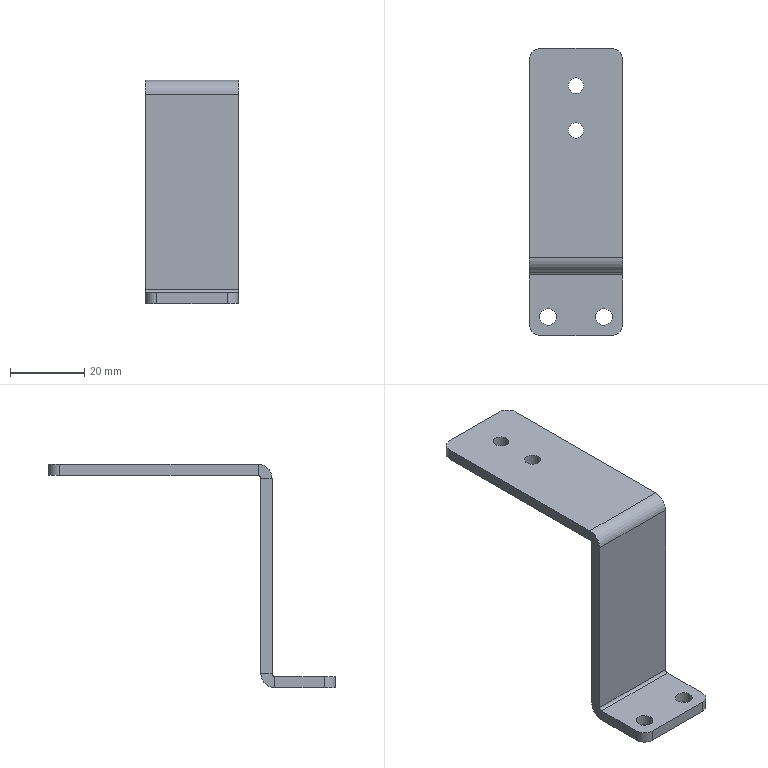Part | SolidWorks | features EdgeFlange 2, HoleWzd 2, Fillet 1, FlatPattern 1, SMBaseFlange 1, SheetMetal 1 | 1 solid | 34 faces | box 25 x 77 x 60 mm | volume 9704 mm3 | plane 18 | cylinder 16 | commonest cylinder face diameters 4.2 x4 4.5 x4 6 x4 1.473 x2 7.473 x2
STEP:
#1=CARTESIAN_POINT('',(2.1,57.,54.));
#2=VERTEX_POINT('',#1);
#3=CARTESIAN_POINT('',(-2.1,57.,54.));
#4=VERTEX_POINT('',#3);
#5=CARTESIAN_POINT('',(0.,57.,54.));
#6=DIRECTION('',(0.,0.,-1.));
#7=DIRECTION('',(-1.,0.,0.));
#8=AXIS2_PLACEMENT_3D('',#5,#6,#7);
#9=CIRCLE('',#8,2.1);
#10=EDGE_CURVE('',#2,#4,#9,.T.);
#11=ORIENTED_EDGE('',*,*,#10,.T.);
#12=CARTESIAN_POINT('',(-2.1,57.,57.));
#13=VERTEX_POINT('',#12);
#14=CARTESIAN_POINT('',(-2.1,57.,57.));
#15=DIRECTION('',(0.,0.,1.));
#16=VECTOR('',#15,1000.);
#17=LINE('',#14,#16);
#18=EDGE_CURVE('',#4,#13,#17,.T.);
#19=ORIENTED_EDGE('',*,*,#18,.T.);
#20=CARTESIAN_POINT('',(2.1,57.,57.));
#21=VERTEX_POINT('',#20);
#22=CARTESIAN_POINT('',(0.,57.,57.));
#23=DIRECTION('',(0.,0.,1.));
#24=DIRECTION('',(1.,0.,0.));
#25=AXIS2_PLACEMENT_3D('',#22,#23,#24);
#26=CIRCLE('',#25,2.1);
#27=EDGE_CURVE('',#13,#21,#26,.T.);
#28=ORIENTED_EDGE('',*,*,#27,.T.);
#29=CARTESIAN_POINT('',(2.1,57.,57.));
#30=DIRECTION('',(0.,0.,1.));
#31=VECTOR('',#30,1000.);
#32=LINE('',#29,#31);
#33=EDGE_CURVE('',#2,#21,#32,.T.);
#34=ORIENTED_EDGE('',*,*,#33,.F.);
#35=EDGE_LOOP('',(#11,#19,#28,#34));
#36=FACE_OUTER_BOUND('',#35,.T.);
#37=CARTESIAN_POINT('',(0.,57.,57.));
#38=DIRECTION('',(0.,0.,1.));
#39=DIRECTION('',(1.,0.,0.));
#40=AXIS2_PLACEMENT_3D('',#37,#38,#39);
#41=CYLINDRICAL_SURFACE('',#40,2.1);
#42=ADVANCED_FACE('',(#36),#41,.F.);
#43=CARTESIAN_POINT('',(2.1,45.,54.));
#44=VERTEX_POINT('',#43);
#45=CARTESIAN_POINT('',(-2.1,45.,54.));
#46=VERTEX_POINT('',#45);
#47=CARTESIAN_POINT('',(0.,45.,54.));
#48=DIRECTION('',(0.,0.,-1.));
#49=DIRECTION('',(-1.,0.,0.));
#50=AXIS2_PLACEMENT_3D('',#47,#48,#49);
#51=CIRCLE('',#50,2.1);
#52=EDGE_CURVE('',#44,#46,#51,.T.);
#53=ORIENTED_EDGE('',*,*,#52,.T.);
#54=CARTESIAN_POINT('',(-2.1,45.,57.));
#55=VERTEX_POINT('',#54);
#56=CARTESIAN_POINT('',(-2.1,45.,57.));
#57=DIRECTION('',(0.,0.,1.));
#58=VECTOR('',#57,1000.);
#59=LINE('',#56,#58);
#60=EDGE_CURVE('',#46,#55,#59,.T.);
#61=ORIENTED_EDGE('',*,*,#60,.T.);
#62=CARTESIAN_POINT('',(2.1,45.,57.));
#63=VERTEX_POINT('',#62);
#64=CARTESIAN_POINT('',(0.,45.,57.));
#65=DIRECTION('',(0.,0.,1.));
#66=DIRECTION('',(1.,0.,0.));
#67=AXIS2_PLACEMENT_3D('',#64,#65,#66);
#68=CIRCLE('',#67,2.1);
#69=EDGE_CURVE('',#55,#63,#68,.T.);
#70=ORIENTED_EDGE('',*,*,#69,.T.);
#71=CARTESIAN_POINT('',(2.1,45.,57.));
#72=DIRECTION('',(0.,0.,1.));
#73=VECTOR('',#72,1000.);
#74=LINE('',#71,#73);
#75=EDGE_CURVE('',#44,#63,#74,.T.);
#76=ORIENTED_EDGE('',*,*,#75,.F.);
#77=EDGE_LOOP('',(#53,#61,#70,#76));
#78=FACE_OUTER_BOUND('',#77,.T.);
#79=CARTESIAN_POINT('',(0.,45.,57.));
#80=DIRECTION('',(0.,0.,1.));
#81=DIRECTION('',(1.,0.,0.));
#82=AXIS2_PLACEMENT_3D('',#79,#80,#81);
#83=CYLINDRICAL_SURFACE('',#82,2.1);
#84=ADVANCED_FACE('',(#78),#83,.F.);
#85=CARTESIAN_POINT('',(-9.75,-5.,-3.));
#86=VERTEX_POINT('',#85);
#87=CARTESIAN_POINT('',(-5.25,-5.,-3.));
#88=VERTEX_POINT('',#87);
#89=CARTESIAN_POINT('',(-7.5,-5.,-3.));
#90=DIRECTION('',(0.,0.,1.));
#91=DIRECTION('',(1.,0.,0.));
#92=AXIS2_PLACEMENT_3D('',#89,#90,#91);
#93=CIRCLE('',#92,2.25);
#94=EDGE_CURVE('',#86,#88,#93,.T.);
#95=ORIENTED_EDGE('',*,*,#94,.F.);
#96=CARTESIAN_POINT('',(-9.75,-5.,0.));
#97=VERTEX_POINT('',#96);
#98=CARTESIAN_POINT('',(-9.75,-5.,0.));
#99=DIRECTION('',(0.,0.,1.));
#100=VECTOR('',#99,1000.);
#101=LINE('',#98,#100);
#102=EDGE_CURVE('',#86,#97,#101,.T.);
#103=ORIENTED_EDGE('',*,*,#102,.T.);
#104=CARTESIAN_POINT('',(-5.25,-5.,0.));
#105=VERTEX_POINT('',#104);
#106=CARTESIAN_POINT('',(-7.5,-5.,0.));
#107=DIRECTION('',(0.,0.,1.));
#108=DIRECTION('',(1.,0.,0.));
#109=AXIS2_PLACEMENT_3D('',#106,#107,#108);
#110=CIRCLE('',#109,2.25);
#111=EDGE_CURVE('',#97,#105,#110,.T.);
#112=ORIENTED_EDGE('',*,*,#111,.T.);
#113=CARTESIAN_POINT('',(-5.25,-5.,0.));
#114=DIRECTION('',(0.,0.,1.));
#115=VECTOR('',#114,1000.);
#116=LINE('',#113,#115);
#117=EDGE_CURVE('',#88,#105,#116,.T.);
#118=ORIENTED_EDGE('',*,*,#117,.F.);
#119=EDGE_LOOP('',(#95,#103,#112,#118));
#120=FACE_OUTER_BOUND('',#119,.T.);
#121=CARTESIAN_POINT('',(-7.5,-5.,0.));
#122=DIRECTION('',(0.,0.,1.));
#123=DIRECTION('',(1.,0.,0.));
#124=AXIS2_PLACEMENT_3D('',#121,#122,#123);
#125=CYLINDRICAL_SURFACE('',#124,2.25);
#126=ADVANCED_FACE('',(#120),#125,.F.);
#127=CARTESIAN_POINT('',(5.25,-5.,-3.));
#128=VERTEX_POINT('',#127);
#129=CARTESIAN_POINT('',(9.75,-5.,-3.));
#130=VERTEX_POINT('',#129);
#131=CARTESIAN_POINT('',(7.5,-5.,-3.));
#132=DIRECTION('',(0.,0.,1.));
#133=DIRECTION('',(1.,0.,0.));
#134=AXIS2_PLACEMENT_3D('',#131,#132,#133);
#135=CIRCLE('',#134,2.25);
#136=EDGE_CURVE('',#128,#130,#135,.T.);
#137=ORIENTED_EDGE('',*,*,#136,.F.);
#138=CARTESIAN_POINT('',(5.25,-5.,0.));
#139=VERTEX_POINT('',#138);
#140=CARTESIAN_POINT('',(5.25,-5.,0.));
#141=DIRECTION('',(0.,0.,1.));
#142=VECTOR('',#141,1000.);
#143=LINE('',#140,#142);
#144=EDGE_CURVE('',#128,#139,#143,.T.);
#145=ORIENTED_EDGE('',*,*,#144,.T.);
#146=CARTESIAN_POINT('',(9.75,-5.,0.));
#147=VERTEX_POINT('',#146);
#148=CARTESIAN_POINT('',(7.5,-5.,0.));
#149=DIRECTION('',(0.,0.,1.));
#150=DIRECTION('',(1.,0.,0.));
#151=AXIS2_PLACEMENT_3D('',#148,#149,#150);
#152=CIRCLE('',#151,2.25);
#153=EDGE_CURVE('',#139,#147,#152,.T.);
#154=ORIENTED_EDGE('',*,*,#153,.T.);
#155=CARTESIAN_POINT('',(9.75,-5.,0.));
#156=DIRECTION('',(0.,0.,1.));
#157=VECTOR('',#156,1000.);
#158=LINE('',#155,#157);
#159=EDGE_CURVE('',#130,#147,#158,.T.);
#160=ORIENTED_EDGE('',*,*,#159,.F.);
#161=EDGE_LOOP('',(#137,#145,#154,#160));
#162=FACE_OUTER_BOUND('',#161,.T.);
#163=CARTESIAN_POINT('',(7.5,-5.,0.));
#164=DIRECTION('',(0.,0.,1.));
#165=DIRECTION('',(1.,0.,0.));
#166=AXIS2_PLACEMENT_3D('',#163,#164,#165);
#167=CYLINDRICAL_SURFACE('',#166,2.25);
#168=ADVANCED_FACE('',(#162),#167,.F.);
#169=CARTESIAN_POINT('',(12.5,10.,53.263));
#170=VERTEX_POINT('',#169);
#171=CARTESIAN_POINT('',(12.5,7.,53.263));
#172=VERTEX_POINT('',#171);
#173=CARTESIAN_POINT('',(12.5,10.,53.263));
#174=DIRECTION('',(0.,-1.,0.));
#175=VECTOR('',#174,1000.);
#176=LINE('',#173,#175);
#177=EDGE_CURVE('',#170,#172,#176,.T.);
#178=ORIENTED_EDGE('',*,*,#177,.T.);
#179=CARTESIAN_POINT('',(12.5,7.,0.7366));
#180=VERTEX_POINT('',#179);
#181=CARTESIAN_POINT('',(12.5,7.,0.));
#182=DIRECTION('',(0.,0.,-1.));
#183=VECTOR('',#182,1000.);
#184=LINE('',#181,#183);
#185=EDGE_CURVE('',#172,#180,#184,.T.);
#186=ORIENTED_EDGE('',*,*,#185,.T.);
#187=CARTESIAN_POINT('',(12.5,10.,0.7366));
#188=VERTEX_POINT('',#187);
#189=CARTESIAN_POINT('',(12.5,10.,0.7366));
#190=DIRECTION('',(0.,1.,0.));
#191=VECTOR('',#190,1000.);
#192=LINE('',#189,#191);
#193=EDGE_CURVE('',#180,#188,#192,.T.);
#194=ORIENTED_EDGE('',*,*,#193,.T.);
#195=CARTESIAN_POINT('',(12.5,10.,0.));
#196=DIRECTION('',(0.,0.,-1.));
#197=VECTOR('',#196,1000.);
#198=LINE('',#195,#197);
#199=EDGE_CURVE('',#170,#188,#198,.T.);
#200=ORIENTED_EDGE('',*,*,#199,.F.);
#201=EDGE_LOOP('',(#178,#186,#194,#200));
#202=FACE_OUTER_BOUND('',#201,.T.);
#203=CARTESIAN_POINT('',(12.5,10.,0.));
#204=DIRECTION('',(-1.,0.,0.));
#205=DIRECTION('',(0.,0.,1.));
#206=AXIS2_PLACEMENT_3D('',#203,#204,#205);
#207=PLANE('',#206);
#208=ADVANCED_FACE('',(#202),#207,.F.);
#209=CARTESIAN_POINT('',(-12.5,10.,53.263));
#210=VERTEX_POINT('',#209);
#211=CARTESIAN_POINT('',(-12.5,7.,53.263));
#212=VERTEX_POINT('',#211);
#213=CARTESIAN_POINT('',(-12.5,10.,53.263));
#214=DIRECTION('',(0.,-1.,0.));
#215=VECTOR('',#214,1000.);
#216=LINE('',#213,#215);
#217=EDGE_CURVE('',#210,#212,#216,.T.);
#218=ORIENTED_EDGE('',*,*,#217,.F.);
#219=CARTESIAN_POINT('',(-12.5,10.,0.7366));
#220=VERTEX_POINT('',#219);
#221=CARTESIAN_POINT('',(-12.5,10.,0.));
#222=DIRECTION('',(0.,0.,1.));
#223=VECTOR('',#222,1000.);
#224=LINE('',#221,#223);
#225=EDGE_CURVE('',#220,#210,#224,.T.);
#226=ORIENTED_EDGE('',*,*,#225,.F.);
#227=CARTESIAN_POINT('',(-12.5,7.,0.7366));
#228=VERTEX_POINT('',#227);
#229=CARTESIAN_POINT('',(-12.5,7.,0.7366));
#230=DIRECTION('',(0.,1.,0.));
#231=VECTOR('',#230,1000.);
#232=LINE('',#229,#231);
#233=EDGE_CURVE('',#228,#220,#232,.T.);
#234=ORIENTED_EDGE('',*,*,#233,.F.);
#235=CARTESIAN_POINT('',(-12.5,7.,57.));
#236=DIRECTION('',(0.,0.,1.));
#237=VECTOR('',#236,1000.);
#238=LINE('',#235,#237);
#239=EDGE_CURVE('',#228,#212,#238,.T.);
#240=ORIENTED_EDGE('',*,*,#239,.T.);
#241=EDGE_LOOP('',(#218,#226,#234,#240));
#242=FACE_OUTER_BOUND('',#241,.T.);
#243=CARTESIAN_POINT('',(-12.5,10.,57.));
#244=DIRECTION('',(1.,0.,0.));
#245=DIRECTION('',(0.,0.,-1.));
#246=AXIS2_PLACEMENT_3D('',#243,#244,#245);
#247=PLANE('',#246);
#248=ADVANCED_FACE('',(#242),#247,.F.);
#249=CARTESIAN_POINT('',(12.5,10.,53.263));
#250=DIRECTION('',(-1.,0.,0.));
#251=VECTOR('',#250,1000.);
#252=LINE('',#249,#251);
#253=EDGE_CURVE('',#170,#210,#252,.T.);
#254=ORIENTED_EDGE('',*,*,#253,.F.);
#255=ORIENTED_EDGE('',*,*,#199,.T.);
#256=CARTESIAN_POINT('',(12.5,10.,0.7366));
#257=DIRECTION('',(1.,0.,0.));
#258=VECTOR('',#257,1000.);
#259=LINE('',#256,#258);
#260=EDGE_CURVE('',#220,#188,#259,.T.);
#261=ORIENTED_EDGE('',*,*,#260,.F.);
#262=ORIENTED_EDGE('',*,*,#225,.T.);
#263=EDGE_LOOP('',(#254,#255,#261,#262));
#264=FACE_OUTER_BOUND('',#263,.T.);
#265=CARTESIAN_POINT('',(0.,10.,0.));
#266=DIRECTION('',(0.,-1.,0.));
#267=DIRECTION('',(0.,0.,-1.));
#268=AXIS2_PLACEMENT_3D('',#265,#266,#267);
#269=PLANE('',#268);
#270=ADVANCED_FACE('',(#264),#269,.F.);
#271=ORIENTED_EDGE('',*,*,#185,.F.);
#272=CARTESIAN_POINT('',(12.5,7.,53.263));
#273=DIRECTION('',(-1.,0.,0.));
#274=VECTOR('',#273,1000.);
#275=LINE('',#272,#274);
#276=EDGE_CURVE('',#172,#212,#275,.T.);
#277=ORIENTED_EDGE('',*,*,#276,.T.);
#278=ORIENTED_EDGE('',*,*,#239,.F.);
#279=CARTESIAN_POINT('',(12.5,7.,0.7366));
#280=DIRECTION('',(-1.,0.,0.));
#281=VECTOR('',#280,1000.);
#282=LINE('',#279,#281);
#283=EDGE_CURVE('',#180,#228,#282,.T.);
#284=ORIENTED_EDGE('',*,*,#283,.F.);
#285=EDGE_LOOP('',(#271,#277,#278,#284));
#286=FACE_OUTER_BOUND('',#285,.T.);
#287=CARTESIAN_POINT('',(0.,7.,0.));
#288=DIRECTION('',(0.,-1.,0.));
#289=DIRECTION('',(0.,0.,-1.));
#290=AXIS2_PLACEMENT_3D('',#287,#288,#289);
#291=PLANE('',#290);
#292=ADVANCED_FACE('',(#286),#291,.T.);
#293=CARTESIAN_POINT('',(-12.5,6.263,-3.));
#294=VERTEX_POINT('',#293);
#295=CARTESIAN_POINT('',(-12.5,-7.,-3.));
#296=VERTEX_POINT('',#295);
#297=CARTESIAN_POINT('',(-12.5,10.,-3.));
#298=DIRECTION('',(0.,-1.,0.));
#299=VECTOR('',#298,1000.);
#300=LINE('',#297,#299);
#301=EDGE_CURVE('',#294,#296,#300,.T.);
#302=ORIENTED_EDGE('',*,*,#301,.T.);
#303=CARTESIAN_POINT('',(-12.5,-7.,0.));
#304=VERTEX_POINT('',#303);
#305=CARTESIAN_POINT('',(-12.5,-7.,-3.));
#306=DIRECTION('',(0.,0.,1.));
#307=VECTOR('',#306,1000.);
#308=LINE('',#305,#307);
#309=EDGE_CURVE('',#296,#304,#308,.T.);
#310=ORIENTED_EDGE('',*,*,#309,.T.);
#311=CARTESIAN_POINT('',(-12.5,6.263,0.));
#312=VERTEX_POINT('',#311);
#313=CARTESIAN_POINT('',(-12.5,10.,0.));
#314=DIRECTION('',(0.,-1.,0.));
#315=VECTOR('',#314,1000.);
#316=LINE('',#313,#315);
#317=EDGE_CURVE('',#312,#304,#316,.T.);
#318=ORIENTED_EDGE('',*,*,#317,.F.);
#319=CARTESIAN_POINT('',(-12.5,6.263,0.));
#320=DIRECTION('',(0.,0.,-1.));
#321=VECTOR('',#320,1000.);
#322=LINE('',#319,#321);
#323=EDGE_CURVE('',#312,#294,#322,.T.);
#324=ORIENTED_EDGE('',*,*,#323,.T.);
#325=EDGE_LOOP('',(#302,#310,#318,#324));
#326=FACE_OUTER_BOUND('',#325,.T.);
#327=CARTESIAN_POINT('',(-12.5,10.,-3.));
#328=DIRECTION('',(-1.,0.,0.));
#329=DIRECTION('',(0.,-1.,0.));
#330=AXIS2_PLACEMENT_3D('',#327,#328,#329);
#331=PLANE('',#330);
#332=ADVANCED_FACE('',(#326),#331,.T.);
#333=CARTESIAN_POINT('',(-7.5,-5.,-3.));
#334=DIRECTION('',(0.,0.,1.));
#335=DIRECTION('',(1.,0.,0.));
#336=AXIS2_PLACEMENT_3D('',#333,#334,#335);
#337=CIRCLE('',#336,2.25);
#338=EDGE_CURVE('',#88,#86,#337,.T.);
#339=ORIENTED_EDGE('',*,*,#338,.T.);
#340=ORIENTED_EDGE('',*,*,#94,.T.);
#341=EDGE_LOOP('',(#339,#340));
#342=FACE_BOUND('',#341,.T.);
#343=CARTESIAN_POINT('',(7.5,-5.,-3.));
#344=DIRECTION('',(0.,0.,1.));
#345=DIRECTION('',(1.,0.,0.));
#346=AXIS2_PLACEMENT_3D('',#343,#344,#345);
#347=CIRCLE('',#346,2.25);
#348=EDGE_CURVE('',#130,#128,#347,.T.);
#349=ORIENTED_EDGE('',*,*,#348,.T.);
#350=ORIENTED_EDGE('',*,*,#136,.T.);
#351=EDGE_LOOP('',(#349,#350));
#352=FACE_BOUND('',#351,.T.);
#353=CARTESIAN_POINT('',(12.5,-7.,-3.));
#354=VERTEX_POINT('',#353);
#355=CARTESIAN_POINT('',(12.5,6.263,-3.));
#356=VERTEX_POINT('',#355);
#357=CARTESIAN_POINT('',(12.5,10.,-3.));
#358=DIRECTION('',(0.,1.,0.));
#359=VECTOR('',#358,1000.);
#360=LINE('',#357,#359);
#361=EDGE_CURVE('',#354,#356,#360,.T.);
#362=ORIENTED_EDGE('',*,*,#361,.F.);
#363=CARTESIAN_POINT('',(9.5,-10.,-3.));
#364=VERTEX_POINT('',#363);
#365=CARTESIAN_POINT('',(9.5,-7.,-3.));
#366=DIRECTION('',(0.,0.,-1.));
#367=DIRECTION('',(1.,0.,0.));
#368=AXIS2_PLACEMENT_3D('',#365,#366,#367);
#369=CIRCLE('',#368,3.);
#370=EDGE_CURVE('',#354,#364,#369,.T.);
#371=ORIENTED_EDGE('',*,*,#370,.T.);
#372=CARTESIAN_POINT('',(-9.5,-10.,-3.));
#373=VERTEX_POINT('',#372);
#374=CARTESIAN_POINT('',(-12.5,-10.,-3.));
#375=DIRECTION('',(1.,0.,0.));
#376=VECTOR('',#375,1000.);
#377=LINE('',#374,#376);
#378=EDGE_CURVE('',#373,#364,#377,.T.);
#379=ORIENTED_EDGE('',*,*,#378,.F.);
#380=CARTESIAN_POINT('',(-9.5,-7.,-3.));
#381=DIRECTION('',(0.,0.,-1.));
#382=DIRECTION('',(1.,0.,0.));
#383=AXIS2_PLACEMENT_3D('',#380,#381,#382);
#384=CIRCLE('',#383,3.);
#385=EDGE_CURVE('',#373,#296,#384,.T.);
#386=ORIENTED_EDGE('',*,*,#385,.T.);
#387=ORIENTED_EDGE('',*,*,#301,.F.);
#388=CARTESIAN_POINT('',(-12.5,6.263,-3.));
#389=DIRECTION('',(1.,0.,0.));
#390=VECTOR('',#389,1000.);
#391=LINE('',#388,#390);
#392=EDGE_CURVE('',#294,#356,#391,.T.);
#393=ORIENTED_EDGE('',*,*,#392,.T.);
#394=EDGE_LOOP('',(#362,#371,#379,#386,#387,#393));
#395=FACE_OUTER_BOUND('',#394,.T.);
#396=CARTESIAN_POINT('',(0.,0.,-3.));
#397=DIRECTION('',(0.,0.,1.));
#398=DIRECTION('',(1.,0.,0.));
#399=AXIS2_PLACEMENT_3D('',#396,#397,#398);
#400=PLANE('',#399);
#401=ADVANCED_FACE('',(#342,#352,#395),#400,.F.);
#402=CARTESIAN_POINT('',(-7.5,-5.,0.));
#403=DIRECTION('',(0.,0.,1.));
#404=DIRECTION('',(1.,0.,0.));
#405=AXIS2_PLACEMENT_3D('',#402,#403,#404);
#406=CIRCLE('',#405,2.25);
#407=EDGE_CURVE('',#105,#97,#406,.T.);
#408=ORIENTED_EDGE('',*,*,#407,.F.);
#409=ORIENTED_EDGE('',*,*,#111,.F.);
#410=EDGE_LOOP('',(#408,#409));
#411=FACE_BOUND('',#410,.T.);
#412=CARTESIAN_POINT('',(7.5,-5.,0.));
#413=DIRECTION('',(0.,0.,1.));
#414=DIRECTION('',(1.,0.,0.));
#415=AXIS2_PLACEMENT_3D('',#412,#413,#414);
#416=CIRCLE('',#415,2.25);
#417=EDGE_CURVE('',#147,#139,#416,.T.);
#418=ORIENTED_EDGE('',*,*,#417,.F.);
#419=ORIENTED_EDGE('',*,*,#153,.F.);
#420=EDGE_LOOP('',(#418,#419));
#421=FACE_BOUND('',#420,.T.);
#422=CARTESIAN_POINT('',(-9.5,-10.,0.));
#423=VERTEX_POINT('',#422);
#424=CARTESIAN_POINT('',(9.5,-10.,0.));
#425=VERTEX_POINT('',#424);
#426=CARTESIAN_POINT('',(-12.5,-10.,0.));
#427=DIRECTION('',(1.,0.,0.));
#428=VECTOR('',#427,1000.);
#429=LINE('',#426,#428);
#430=EDGE_CURVE('',#423,#425,#429,.T.);
#431=ORIENTED_EDGE('',*,*,#430,.T.);
#432=CARTESIAN_POINT('',(12.5,-7.,0.));
#433=VERTEX_POINT('',#432);
#434=CARTESIAN_POINT('',(9.5,-7.,0.));
#435=DIRECTION('',(0.,0.,1.));
#436=DIRECTION('',(1.,0.,0.));
#437=AXIS2_PLACEMENT_3D('',#434,#435,#436);
#438=CIRCLE('',#437,3.);
#439=EDGE_CURVE('',#425,#433,#438,.T.);
#440=ORIENTED_EDGE('',*,*,#439,.T.);
#441=CARTESIAN_POINT('',(12.5,6.263,0.));
#442=VERTEX_POINT('',#441);
#443=CARTESIAN_POINT('',(12.5,10.,0.));
#444=DIRECTION('',(0.,1.,0.));
#445=VECTOR('',#444,1000.);
#446=LINE('',#443,#445);
#447=EDGE_CURVE('',#433,#442,#446,.T.);
#448=ORIENTED_EDGE('',*,*,#447,.T.);
#449=CARTESIAN_POINT('',(-12.5,6.263,0.));
#450=DIRECTION('',(1.,0.,0.));
#451=VECTOR('',#450,1000.);
#452=LINE('',#449,#451);
#453=EDGE_CURVE('',#312,#442,#452,.T.);
#454=ORIENTED_EDGE('',*,*,#453,.F.);
#455=ORIENTED_EDGE('',*,*,#317,.T.);
#456=CARTESIAN_POINT('',(-9.5,-7.,0.));
#457=DIRECTION('',(0.,0.,1.));
#458=DIRECTION('',(1.,0.,0.));
#459=AXIS2_PLACEMENT_3D('',#456,#457,#458);
#460=CIRCLE('',#459,3.);
#461=EDGE_CURVE('',#304,#423,#460,.T.);
#462=ORIENTED_EDGE('',*,*,#461,.T.);
#463=EDGE_LOOP('',(#431,#440,#448,#454,#455,#462));
#464=FACE_OUTER_BOUND('',#463,.T.);
#465=CARTESIAN_POINT('',(0.,0.,0.));
#466=DIRECTION('',(0.,0.,1.));
#467=DIRECTION('',(1.,0.,0.));
#468=AXIS2_PLACEMENT_3D('',#465,#466,#467);
#469=PLANE('',#468);
#470=ADVANCED_FACE('',(#411,#421,#464),#469,.T.);
#471=ORIENTED_EDGE('',*,*,#447,.F.);
#472=CARTESIAN_POINT('',(12.5,-7.,-3.));
#473=DIRECTION('',(0.,0.,-1.));
#474=VECTOR('',#473,1000.);
#475=LINE('',#472,#474);
#476=EDGE_CURVE('',#433,#354,#475,.T.);
#477=ORIENTED_EDGE('',*,*,#476,.T.);
#478=ORIENTED_EDGE('',*,*,#361,.T.);
#479=CARTESIAN_POINT('',(12.5,6.263,0.));
#480=DIRECTION('',(0.,0.,-1.));
#481=VECTOR('',#480,1000.);
#482=LINE('',#479,#481);
#483=EDGE_CURVE('',#442,#356,#482,.T.);
#484=ORIENTED_EDGE('',*,*,#483,.F.);
#485=EDGE_LOOP('',(#471,#477,#478,#484));
#486=FACE_OUTER_BOUND('',#485,.T.);
#487=CARTESIAN_POINT('',(12.5,10.,-3.));
#488=DIRECTION('',(1.,0.,0.));
#489=DIRECTION('',(0.,1.,0.));
#490=AXIS2_PLACEMENT_3D('',#487,#488,#489);
#491=PLANE('',#490);
#492=ADVANCED_FACE('',(#486),#491,.T.);
#493=ORIENTED_EDGE('',*,*,#378,.T.);
#494=CARTESIAN_POINT('',(9.5,-10.,-3.));
#495=DIRECTION('',(0.,0.,1.));
#496=VECTOR('',#495,1000.);
#497=LINE('',#494,#496);
#498=EDGE_CURVE('',#364,#425,#497,.T.);
#499=ORIENTED_EDGE('',*,*,#498,.T.);
#500=ORIENTED_EDGE('',*,*,#430,.F.);
#501=CARTESIAN_POINT('',(-9.5,-10.,-3.));
#502=DIRECTION('',(0.,0.,-1.));
#503=VECTOR('',#502,1000.);
#504=LINE('',#501,#503);
#505=EDGE_CURVE('',#423,#373,#504,.T.);
#506=ORIENTED_EDGE('',*,*,#505,.T.);
#507=EDGE_LOOP('',(#493,#499,#500,#506));
#508=FACE_OUTER_BOUND('',#507,.T.);
#509=CARTESIAN_POINT('',(-12.5,-10.,-3.));
#510=DIRECTION('',(0.,-1.,0.));
#511=DIRECTION('',(0.,0.,-1.));
#512=AXIS2_PLACEMENT_3D('',#509,#510,#511);
#513=PLANE('',#512);
#514=ADVANCED_FACE('',(#508),#513,.T.);
#515=ORIENTED_EDGE('',*,*,#193,.F.);
#516=CARTESIAN_POINT('',(12.5,6.263,0.7366));
#517=DIRECTION('',(1.,0.,0.));
#518=DIRECTION('',(0.,0.,1.));
#519=AXIS2_PLACEMENT_3D('',#516,#517,#518);
#520=CIRCLE('',#519,0.7366);
#521=EDGE_CURVE('',#442,#180,#520,.T.);
#522=ORIENTED_EDGE('',*,*,#521,.F.);
#523=ORIENTED_EDGE('',*,*,#483,.T.);
#524=CARTESIAN_POINT('',(12.5,6.263,0.7366));
#525=DIRECTION('',(1.,0.,0.));
#526=DIRECTION('',(0.,0.,1.));
#527=AXIS2_PLACEMENT_3D('',#524,#525,#526);
#528=CIRCLE('',#527,3.737);
#529=EDGE_CURVE('',#356,#188,#528,.T.);
#530=ORIENTED_EDGE('',*,*,#529,.T.);
#531=EDGE_LOOP('',(#515,#522,#523,#530));
#532=FACE_OUTER_BOUND('',#531,.T.);
#533=CARTESIAN_POINT('',(12.5,6.263,0.7366));
#534=DIRECTION('',(1.,0.,0.));
#535=DIRECTION('',(0.,0.,-1.));
#536=AXIS2_PLACEMENT_3D('',#533,#534,#535);
#537=PLANE('',#536);
#538=ADVANCED_FACE('',(#532),#537,.T.);
#539=CARTESIAN_POINT('',(-12.5,6.263,0.7366));
#540=DIRECTION('',(-1.,0.,0.));
#541=DIRECTION('',(0.,0.,1.));
#542=AXIS2_PLACEMENT_3D('',#539,#540,#541);
#543=CIRCLE('',#542,0.7366);
#544=EDGE_CURVE('',#228,#312,#543,.T.);
#545=ORIENTED_EDGE('',*,*,#544,.F.);
#546=ORIENTED_EDGE('',*,*,#233,.T.);
#547=CARTESIAN_POINT('',(-12.5,6.263,0.7366));
#548=DIRECTION('',(-1.,0.,0.));
#549=DIRECTION('',(0.,0.,1.));
#550=AXIS2_PLACEMENT_3D('',#547,#548,#549);
#551=CIRCLE('',#550,3.737);
#552=EDGE_CURVE('',#220,#294,#551,.T.);
#553=ORIENTED_EDGE('',*,*,#552,.T.);
#554=ORIENTED_EDGE('',*,*,#323,.F.);
#555=EDGE_LOOP('',(#545,#546,#553,#554));
#556=FACE_OUTER_BOUND('',#555,.T.);
#557=CARTESIAN_POINT('',(-12.5,6.263,0.7366));
#558=DIRECTION('',(1.,0.,0.));
#559=DIRECTION('',(0.,0.,-1.));
#560=AXIS2_PLACEMENT_3D('',#557,#558,#559);
#561=PLANE('',#560);
#562=ADVANCED_FACE('',(#556),#561,.F.);
#563=ORIENTED_EDGE('',*,*,#392,.F.);
#564=ORIENTED_EDGE('',*,*,#552,.F.);
#565=ORIENTED_EDGE('',*,*,#260,.T.);
#566=ORIENTED_EDGE('',*,*,#529,.F.);
#567=EDGE_LOOP('',(#563,#564,#565,#566));
#568=FACE_OUTER_BOUND('',#567,.T.);
#569=CARTESIAN_POINT('',(-12.5,6.263,0.7366));
#570=DIRECTION('',(-1.,0.,0.));
#571=DIRECTION('',(0.,1.,0.));
#572=AXIS2_PLACEMENT_3D('',#569,#570,#571);
#573=CYLINDRICAL_SURFACE('',#572,3.737);
#574=ADVANCED_FACE('',(#568),#573,.T.);
#575=ORIENTED_EDGE('',*,*,#453,.T.);
#576=ORIENTED_EDGE('',*,*,#521,.T.);
#577=ORIENTED_EDGE('',*,*,#283,.T.);
#578=ORIENTED_EDGE('',*,*,#544,.T.);
#579=EDGE_LOOP('',(#575,#576,#577,#578));
#580=FACE_OUTER_BOUND('',#579,.T.);
#581=CARTESIAN_POINT('',(-12.5,6.263,0.7366));
#582=DIRECTION('',(-1.,0.,0.));
#583=DIRECTION('',(0.,1.,0.));
#584=AXIS2_PLACEMENT_3D('',#581,#582,#583);
#585=CYLINDRICAL_SURFACE('',#584,0.7366);
#586=ADVANCED_FACE('',(#580),#585,.F.);
#587=CARTESIAN_POINT('',(-12.5,10.737,54.));
#588=VERTEX_POINT('',#587);
#589=CARTESIAN_POINT('',(-12.5,10.737,57.));
#590=VERTEX_POINT('',#589);
#591=CARTESIAN_POINT('',(-12.5,10.737,57.));
#592=DIRECTION('',(0.,0.,1.));
#593=VECTOR('',#592,1000.);
#594=LINE('',#591,#593);
#595=EDGE_CURVE('',#588,#590,#594,.T.);
#596=ORIENTED_EDGE('',*,*,#595,.F.);
#597=CARTESIAN_POINT('',(-12.5,10.737,53.263));
#598=DIRECTION('',(-1.,0.,0.));
#599=DIRECTION('',(0.,0.,-1.));
#600=AXIS2_PLACEMENT_3D('',#597,#598,#599);
#601=CIRCLE('',#600,0.7366);
#602=EDGE_CURVE('',#210,#588,#601,.T.);
#603=ORIENTED_EDGE('',*,*,#602,.F.);
#604=ORIENTED_EDGE('',*,*,#217,.T.);
#605=CARTESIAN_POINT('',(-12.5,10.737,53.263));
#606=DIRECTION('',(-1.,0.,0.));
#607=DIRECTION('',(0.,0.,-1.));
#608=AXIS2_PLACEMENT_3D('',#605,#606,#607);
#609=CIRCLE('',#608,3.737);
#610=EDGE_CURVE('',#212,#590,#609,.T.);
#611=ORIENTED_EDGE('',*,*,#610,.T.);
#612=EDGE_LOOP('',(#596,#603,#604,#611));
#613=FACE_OUTER_BOUND('',#612,.T.);
#614=CARTESIAN_POINT('',(-12.5,10.737,53.263));
#615=DIRECTION('',(-1.,0.,0.));
#616=DIRECTION('',(0.,0.,1.));
#617=AXIS2_PLACEMENT_3D('',#614,#615,#616);
#618=PLANE('',#617);
#619=ADVANCED_FACE('',(#613),#618,.T.);
#620=CARTESIAN_POINT('',(12.5,10.737,54.));
#621=VERTEX_POINT('',#620);
#622=CARTESIAN_POINT('',(12.5,10.737,53.263));
#623=DIRECTION('',(1.,0.,0.));
#624=DIRECTION('',(0.,0.,-1.));
#625=AXIS2_PLACEMENT_3D('',#622,#623,#624);
#626=CIRCLE('',#625,0.7366);
#627=EDGE_CURVE('',#621,#170,#626,.T.);
#628=ORIENTED_EDGE('',*,*,#627,.F.);
#629=CARTESIAN_POINT('',(12.5,10.737,57.));
#630=VERTEX_POINT('',#629);
#631=CARTESIAN_POINT('',(12.5,10.737,54.));
#632=DIRECTION('',(0.,0.,1.));
#633=VECTOR('',#632,1000.);
#634=LINE('',#631,#633);
#635=EDGE_CURVE('',#621,#630,#634,.T.);
#636=ORIENTED_EDGE('',*,*,#635,.T.);
#637=CARTESIAN_POINT('',(12.5,10.737,53.263));
#638=DIRECTION('',(1.,0.,0.));
#639=DIRECTION('',(0.,0.,-1.));
#640=AXIS2_PLACEMENT_3D('',#637,#638,#639);
#641=CIRCLE('',#640,3.737);
#642=EDGE_CURVE('',#630,#172,#641,.T.);
#643=ORIENTED_EDGE('',*,*,#642,.T.);
#644=ORIENTED_EDGE('',*,*,#177,.F.);
#645=EDGE_LOOP('',(#628,#636,#643,#644));
#646=FACE_OUTER_BOUND('',#645,.T.);
#647=CARTESIAN_POINT('',(12.5,10.737,53.263));
#648=DIRECTION('',(-1.,0.,0.));
#649=DIRECTION('',(0.,0.,1.));
#650=AXIS2_PLACEMENT_3D('',#647,#648,#649);
#651=PLANE('',#650);
#652=ADVANCED_FACE('',(#646),#651,.F.);
#653=ORIENTED_EDGE('',*,*,#276,.F.);
#654=ORIENTED_EDGE('',*,*,#642,.F.);
#655=CARTESIAN_POINT('',(-12.5,10.737,57.));
#656=DIRECTION('',(-1.,0.,0.));
#657=VECTOR('',#656,1000.);
#658=LINE('',#655,#657);
#659=EDGE_CURVE('',#630,#590,#658,.T.);
#660=ORIENTED_EDGE('',*,*,#659,.T.);
#661=ORIENTED_EDGE('',*,*,#610,.F.);
#662=EDGE_LOOP('',(#653,#654,#660,#661));
#663=FACE_OUTER_BOUND('',#662,.T.);
#664=CARTESIAN_POINT('',(12.5,10.737,53.263));
#665=DIRECTION('',(1.,0.,0.));
#666=DIRECTION('',(0.,0.,1.));
#667=AXIS2_PLACEMENT_3D('',#664,#665,#666);
#668=CYLINDRICAL_SURFACE('',#667,3.737);
#669=ADVANCED_FACE('',(#663),#668,.T.);
#670=ORIENTED_EDGE('',*,*,#253,.T.);
#671=ORIENTED_EDGE('',*,*,#602,.T.);
#672=CARTESIAN_POINT('',(-12.5,10.737,54.));
#673=DIRECTION('',(1.,0.,0.));
#674=VECTOR('',#673,1000.);
#675=LINE('',#672,#674);
#676=EDGE_CURVE('',#588,#621,#675,.T.);
#677=ORIENTED_EDGE('',*,*,#676,.T.);
#678=ORIENTED_EDGE('',*,*,#627,.T.);
#679=EDGE_LOOP('',(#670,#671,#677,#678));
#680=FACE_OUTER_BOUND('',#679,.T.);
#681=CARTESIAN_POINT('',(12.5,10.737,53.263));
#682=DIRECTION('',(1.,0.,0.));
#683=DIRECTION('',(0.,0.,1.));
#684=AXIS2_PLACEMENT_3D('',#681,#682,#683);
#685=CYLINDRICAL_SURFACE('',#684,0.7366);
#686=ADVANCED_FACE('',(#680),#685,.F.);
#687=CARTESIAN_POINT('',(-12.5,64.,57.));
#688=VERTEX_POINT('',#687);
#689=CARTESIAN_POINT('',(-12.5,0.,57.));
#690=DIRECTION('',(0.,-1.,0.));
#691=VECTOR('',#690,1000.);
#692=LINE('',#689,#691);
#693=EDGE_CURVE('',#688,#590,#692,.T.);
#694=ORIENTED_EDGE('',*,*,#693,.F.);
#695=CARTESIAN_POINT('',(-12.5,64.,54.));
#696=VERTEX_POINT('',#695);
#697=CARTESIAN_POINT('',(-12.5,64.,57.));
#698=DIRECTION('',(0.,0.,-1.));
#699=VECTOR('',#698,1000.);
#700=LINE('',#697,#699);
#701=EDGE_CURVE('',#688,#696,#700,.T.);
#702=ORIENTED_EDGE('',*,*,#701,.T.);
#703=CARTESIAN_POINT('',(-12.5,10.,54.));
#704=DIRECTION('',(0.,-1.,0.));
#705=VECTOR('',#704,1000.);
#706=LINE('',#703,#705);
#707=EDGE_CURVE('',#696,#588,#706,.T.);
#708=ORIENTED_EDGE('',*,*,#707,.T.);
#709=ORIENTED_EDGE('',*,*,#595,.T.);
#710=EDGE_LOOP('',(#694,#702,#708,#709));
#711=FACE_OUTER_BOUND('',#710,.T.);
#712=CARTESIAN_POINT('',(-12.5,10.,57.));
#713=DIRECTION('',(1.,0.,0.));
#714=DIRECTION('',(0.,0.,-1.));
#715=AXIS2_PLACEMENT_3D('',#712,#713,#714);
#716=PLANE('',#715);
#717=ADVANCED_FACE('',(#711),#716,.F.);
#718=CARTESIAN_POINT('',(12.5,64.,54.));
#719=VERTEX_POINT('',#718);
#720=CARTESIAN_POINT('',(12.5,67.,54.));
#721=DIRECTION('',(0.,1.,0.));
#722=VECTOR('',#721,1000.);
#723=LINE('',#720,#722);
#724=EDGE_CURVE('',#621,#719,#723,.T.);
#725=ORIENTED_EDGE('',*,*,#724,.T.);
#726=CARTESIAN_POINT('',(12.5,64.,57.));
#727=VERTEX_POINT('',#726);
#728=CARTESIAN_POINT('',(12.5,64.,57.));
#729=DIRECTION('',(0.,0.,1.));
#730=VECTOR('',#729,1000.);
#731=LINE('',#728,#730);
#732=EDGE_CURVE('',#719,#727,#731,.T.);
#733=ORIENTED_EDGE('',*,*,#732,.T.);
#734=CARTESIAN_POINT('',(12.5,0.,57.));
#735=DIRECTION('',(0.,1.,0.));
#736=VECTOR('',#735,1000.);
#737=LINE('',#734,#736);
#738=EDGE_CURVE('',#630,#727,#737,.T.);
#739=ORIENTED_EDGE('',*,*,#738,.F.);
#740=ORIENTED_EDGE('',*,*,#635,.F.);
#741=EDGE_LOOP('',(#725,#733,#739,#740));
#742=FACE_OUTER_BOUND('',#741,.T.);
#743=CARTESIAN_POINT('',(12.5,67.,57.));
#744=DIRECTION('',(-1.,0.,0.));
#745=DIRECTION('',(0.,0.,1.));
#746=AXIS2_PLACEMENT_3D('',#743,#744,#745);
#747=PLANE('',#746);
#748=ADVANCED_FACE('',(#742),#747,.F.);
#749=CARTESIAN_POINT('',(0.,57.,57.));
#750=DIRECTION('',(0.,0.,1.));
#751=DIRECTION('',(1.,0.,0.));
#752=AXIS2_PLACEMENT_3D('',#749,#750,#751);
#753=CIRCLE('',#752,2.1);
#754=EDGE_CURVE('',#21,#13,#753,.T.);
#755=ORIENTED_EDGE('',*,*,#754,.F.);
#756=ORIENTED_EDGE('',*,*,#27,.F.);
#757=EDGE_LOOP('',(#755,#756));
#758=FACE_BOUND('',#757,.T.);
#759=CARTESIAN_POINT('',(0.,45.,57.));
#760=DIRECTION('',(0.,0.,1.));
#761=DIRECTION('',(1.,0.,0.));
#762=AXIS2_PLACEMENT_3D('',#759,#760,#761);
#763=CIRCLE('',#762,2.1);
#764=EDGE_CURVE('',#63,#55,#763,.T.);
#765=ORIENTED_EDGE('',*,*,#764,.F.);
#766=ORIENTED_EDGE('',*,*,#69,.F.);
#767=EDGE_LOOP('',(#765,#766));
#768=FACE_BOUND('',#767,.T.);
#769=ORIENTED_EDGE('',*,*,#738,.T.);
#770=CARTESIAN_POINT('',(9.5,67.,57.));
#771=VERTEX_POINT('',#770);
#772=CARTESIAN_POINT('',(9.5,64.,57.));
#773=DIRECTION('',(0.,0.,1.));
#774=DIRECTION('',(-1.,0.,0.));
#775=AXIS2_PLACEMENT_3D('',#772,#773,#774);
#776=CIRCLE('',#775,3.);
#777=EDGE_CURVE('',#727,#771,#776,.T.);
#778=ORIENTED_EDGE('',*,*,#777,.T.);
#779=CARTESIAN_POINT('',(-9.5,67.,57.));
#780=VERTEX_POINT('',#779);
#781=CARTESIAN_POINT('',(0.,67.,57.));
#782=DIRECTION('',(-1.,0.,0.));
#783=VECTOR('',#782,1000.);
#784=LINE('',#781,#783);
#785=EDGE_CURVE('',#771,#780,#784,.T.);
#786=ORIENTED_EDGE('',*,*,#785,.T.);
#787=CARTESIAN_POINT('',(-9.5,64.,57.));
#788=DIRECTION('',(0.,0.,1.));
#789=DIRECTION('',(-1.,0.,0.));
#790=AXIS2_PLACEMENT_3D('',#787,#788,#789);
#791=CIRCLE('',#790,3.);
#792=EDGE_CURVE('',#780,#688,#791,.T.);
#793=ORIENTED_EDGE('',*,*,#792,.T.);
#794=ORIENTED_EDGE('',*,*,#693,.T.);
#795=ORIENTED_EDGE('',*,*,#659,.F.);
#796=EDGE_LOOP('',(#769,#778,#786,#793,#794,#795));
#797=FACE_OUTER_BOUND('',#796,.T.);
#798=CARTESIAN_POINT('',(0.,0.,57.));
#799=DIRECTION('',(0.,0.,-1.));
#800=DIRECTION('',(-1.,0.,0.));
#801=AXIS2_PLACEMENT_3D('',#798,#799,#800);
#802=PLANE('',#801);
#803=ADVANCED_FACE('',(#758,#768,#797),#802,.F.);
#804=ORIENTED_EDGE('',*,*,#10,.F.);
#805=CARTESIAN_POINT('',(0.,57.,54.));
#806=DIRECTION('',(0.,0.,-1.));
#807=DIRECTION('',(-1.,0.,0.));
#808=AXIS2_PLACEMENT_3D('',#805,#806,#807);
#809=CIRCLE('',#808,2.1);
#810=EDGE_CURVE('',#4,#2,#809,.T.);
#811=ORIENTED_EDGE('',*,*,#810,.F.);
#812=EDGE_LOOP('',(#804,#811));
#813=FACE_BOUND('',#812,.T.);
#814=ORIENTED_EDGE('',*,*,#52,.F.);
#815=CARTESIAN_POINT('',(0.,45.,54.));
#816=DIRECTION('',(0.,0.,-1.));
#817=DIRECTION('',(-1.,0.,0.));
#818=AXIS2_PLACEMENT_3D('',#815,#816,#817);
#819=CIRCLE('',#818,2.1);
#820=EDGE_CURVE('',#46,#44,#819,.T.);
#821=ORIENTED_EDGE('',*,*,#820,.F.);
#822=EDGE_LOOP('',(#814,#821));
#823=FACE_BOUND('',#822,.T.);
#824=CARTESIAN_POINT('',(9.5,67.,54.));
#825=VERTEX_POINT('',#824);
#826=CARTESIAN_POINT('',(-9.5,67.,54.));
#827=VERTEX_POINT('',#826);
#828=CARTESIAN_POINT('',(-12.5,67.,54.));
#829=DIRECTION('',(-1.,0.,0.));
#830=VECTOR('',#829,1000.);
#831=LINE('',#828,#830);
#832=EDGE_CURVE('',#825,#827,#831,.T.);
#833=ORIENTED_EDGE('',*,*,#832,.F.);
#834=CARTESIAN_POINT('',(9.5,64.,54.));
#835=DIRECTION('',(0.,0.,-1.));
#836=DIRECTION('',(-1.,0.,0.));
#837=AXIS2_PLACEMENT_3D('',#834,#835,#836);
#838=CIRCLE('',#837,3.);
#839=EDGE_CURVE('',#825,#719,#838,.T.);
#840=ORIENTED_EDGE('',*,*,#839,.T.);
#841=ORIENTED_EDGE('',*,*,#724,.F.);
#842=ORIENTED_EDGE('',*,*,#676,.F.);
#843=ORIENTED_EDGE('',*,*,#707,.F.);
#844=CARTESIAN_POINT('',(-9.5,64.,54.));
#845=DIRECTION('',(0.,0.,-1.));
#846=DIRECTION('',(-1.,0.,0.));
#847=AXIS2_PLACEMENT_3D('',#844,#845,#846);
#848=CIRCLE('',#847,3.);
#849=EDGE_CURVE('',#696,#827,#848,.T.);
#850=ORIENTED_EDGE('',*,*,#849,.T.);
#851=EDGE_LOOP('',(#833,#840,#841,#842,#843,#850));
#852=FACE_OUTER_BOUND('',#851,.T.);
#853=CARTESIAN_POINT('',(0.,0.,54.));
#854=DIRECTION('',(0.,0.,-1.));
#855=DIRECTION('',(-1.,0.,0.));
#856=AXIS2_PLACEMENT_3D('',#853,#854,#855);
#857=PLANE('',#856);
#858=ADVANCED_FACE('',(#813,#823,#852),#857,.T.);
#859=ORIENTED_EDGE('',*,*,#785,.F.);
#860=CARTESIAN_POINT('',(9.5,67.,57.));
#861=DIRECTION('',(0.,0.,-1.));
#862=VECTOR('',#861,1000.);
#863=LINE('',#860,#862);
#864=EDGE_CURVE('',#771,#825,#863,.T.);
#865=ORIENTED_EDGE('',*,*,#864,.T.);
#866=ORIENTED_EDGE('',*,*,#832,.T.);
#867=CARTESIAN_POINT('',(-9.5,67.,57.));
#868=DIRECTION('',(0.,0.,1.));
#869=VECTOR('',#868,1000.);
#870=LINE('',#867,#869);
#871=EDGE_CURVE('',#827,#780,#870,.T.);
#872=ORIENTED_EDGE('',*,*,#871,.T.);
#873=EDGE_LOOP('',(#859,#865,#866,#872));
#874=FACE_OUTER_BOUND('',#873,.T.);
#875=CARTESIAN_POINT('',(-12.5,67.,57.));
#876=DIRECTION('',(0.,-1.,0.));
#877=DIRECTION('',(0.,0.,-1.));
#878=AXIS2_PLACEMENT_3D('',#875,#876,#877);
#879=PLANE('',#878);
#880=ADVANCED_FACE('',(#874),#879,.F.);
#881=ORIENTED_EDGE('',*,*,#144,.F.);
#882=ORIENTED_EDGE('',*,*,#348,.F.);
#883=ORIENTED_EDGE('',*,*,#159,.T.);
#884=ORIENTED_EDGE('',*,*,#417,.T.);
#885=EDGE_LOOP('',(#881,#882,#883,#884));
#886=FACE_OUTER_BOUND('',#885,.T.);
#887=CARTESIAN_POINT('',(7.5,-5.,0.));
#888=DIRECTION('',(0.,0.,1.));
#889=DIRECTION('',(1.,0.,0.));
#890=AXIS2_PLACEMENT_3D('',#887,#888,#889);
#891=CYLINDRICAL_SURFACE('',#890,2.25);
#892=ADVANCED_FACE('',(#886),#891,.F.);
#893=ORIENTED_EDGE('',*,*,#102,.F.);
#894=ORIENTED_EDGE('',*,*,#338,.F.);
#895=ORIENTED_EDGE('',*,*,#117,.T.);
#896=ORIENTED_EDGE('',*,*,#407,.T.);
#897=EDGE_LOOP('',(#893,#894,#895,#896));
#898=FACE_OUTER_BOUND('',#897,.T.);
#899=CARTESIAN_POINT('',(-7.5,-5.,0.));
#900=DIRECTION('',(0.,0.,1.));
#901=DIRECTION('',(1.,0.,0.));
#902=AXIS2_PLACEMENT_3D('',#899,#900,#901);
#903=CYLINDRICAL_SURFACE('',#902,2.25);
#904=ADVANCED_FACE('',(#898),#903,.F.);
#905=ORIENTED_EDGE('',*,*,#60,.F.);
#906=ORIENTED_EDGE('',*,*,#820,.T.);
#907=ORIENTED_EDGE('',*,*,#75,.T.);
#908=ORIENTED_EDGE('',*,*,#764,.T.);
#909=EDGE_LOOP('',(#905,#906,#907,#908));
#910=FACE_OUTER_BOUND('',#909,.T.);
#911=CARTESIAN_POINT('',(0.,45.,57.));
#912=DIRECTION('',(0.,0.,1.));
#913=DIRECTION('',(1.,0.,0.));
#914=AXIS2_PLACEMENT_3D('',#911,#912,#913);
#915=CYLINDRICAL_SURFACE('',#914,2.1);
#916=ADVANCED_FACE('',(#910),#915,.F.);
#917=ORIENTED_EDGE('',*,*,#18,.F.);
#918=ORIENTED_EDGE('',*,*,#810,.T.);
#919=ORIENTED_EDGE('',*,*,#33,.T.);
#920=ORIENTED_EDGE('',*,*,#754,.T.);
#921=EDGE_LOOP('',(#917,#918,#919,#920));
#922=FACE_OUTER_BOUND('',#921,.T.);
#923=CARTESIAN_POINT('',(0.,57.,57.));
#924=DIRECTION('',(0.,0.,1.));
#925=DIRECTION('',(1.,0.,0.));
#926=AXIS2_PLACEMENT_3D('',#923,#924,#925);
#927=CYLINDRICAL_SURFACE('',#926,2.1);
#928=ADVANCED_FACE('',(#922),#927,.F.);
#929=ORIENTED_EDGE('',*,*,#777,.F.);
#930=ORIENTED_EDGE('',*,*,#732,.F.);
#931=ORIENTED_EDGE('',*,*,#839,.F.);
#932=ORIENTED_EDGE('',*,*,#864,.F.);
#933=EDGE_LOOP('',(#929,#930,#931,#932));
#934=FACE_OUTER_BOUND('',#933,.T.);
#935=CARTESIAN_POINT('',(9.5,64.,57.));
#936=DIRECTION('',(0.,0.,-1.));
#937=DIRECTION('',(-1.,0.,0.));
#938=AXIS2_PLACEMENT_3D('',#935,#936,#937);
#939=CYLINDRICAL_SURFACE('',#938,3.);
#940=ADVANCED_FACE('',(#934),#939,.T.);
#941=ORIENTED_EDGE('',*,*,#792,.F.);
#942=ORIENTED_EDGE('',*,*,#871,.F.);
#943=ORIENTED_EDGE('',*,*,#849,.F.);
#944=ORIENTED_EDGE('',*,*,#701,.F.);
#945=EDGE_LOOP('',(#941,#942,#943,#944));
#946=FACE_OUTER_BOUND('',#945,.T.);
#947=CARTESIAN_POINT('',(-9.5,64.,57.));
#948=DIRECTION('',(0.,0.,-1.));
#949=DIRECTION('',(-1.,0.,0.));
#950=AXIS2_PLACEMENT_3D('',#947,#948,#949);
#951=CYLINDRICAL_SURFACE('',#950,3.);
#952=ADVANCED_FACE('',(#946),#951,.T.);
#953=ORIENTED_EDGE('',*,*,#370,.F.);
#954=ORIENTED_EDGE('',*,*,#476,.F.);
#955=ORIENTED_EDGE('',*,*,#439,.F.);
#956=ORIENTED_EDGE('',*,*,#498,.F.);
#957=EDGE_LOOP('',(#953,#954,#955,#956));
#958=FACE_OUTER_BOUND('',#957,.T.);
#959=CARTESIAN_POINT('',(9.5,-7.,-3.));
#960=DIRECTION('',(0.,0.,1.));
#961=DIRECTION('',(1.,0.,0.));
#962=AXIS2_PLACEMENT_3D('',#959,#960,#961);
#963=CYLINDRICAL_SURFACE('',#962,3.);
#964=ADVANCED_FACE('',(#958),#963,.T.);
#965=ORIENTED_EDGE('',*,*,#385,.F.);
#966=ORIENTED_EDGE('',*,*,#505,.F.);
#967=ORIENTED_EDGE('',*,*,#461,.F.);
#968=ORIENTED_EDGE('',*,*,#309,.F.);
#969=EDGE_LOOP('',(#965,#966,#967,#968));
#970=FACE_OUTER_BOUND('',#969,.T.);
#971=CARTESIAN_POINT('',(-9.5,-7.,-3.));
#972=DIRECTION('',(0.,0.,1.));
#973=DIRECTION('',(1.,0.,0.));
#974=AXIS2_PLACEMENT_3D('',#971,#972,#973);
#975=CYLINDRICAL_SURFACE('',#974,3.);
#976=ADVANCED_FACE('',(#970),#975,.T.);
#977=CLOSED_SHELL('',(#42,#84,#126,#168,#208,#248,#270,#292,#332,#401,#470,#492,#514,#538,#562,#574,#586,#619,#652,#669,#686,#717,#748,#803,#858,#880,#892,#904,#916,#928,#940,#952,#964,#976));
#978=MANIFOLD_SOLID_BREP('',#977);
#979=CARTESIAN_POINT('',(0.,0.,0.));
#980=DIRECTION('',(0.,0.,1.));
#981=DIRECTION('',(1.,0.,0.));
#982=AXIS2_PLACEMENT_3D('',#979,#980,#981);
#983=(LENGTH_UNIT()NAMED_UNIT(*)SI_UNIT(.MILLI.,.METRE.));
#984=UNCERTAINTY_MEASURE_WITH_UNIT(LENGTH_MEASURE(0.00001),#983,'','');
#985=(NAMED_UNIT(*)PLANE_ANGLE_UNIT()SI_UNIT($,.RADIAN.));
#986=(NAMED_UNIT(*)SI_UNIT($,.STERADIAN.)SOLID_ANGLE_UNIT());
#987=(GEOMETRIC_REPRESENTATION_CONTEXT(3)GLOBAL_UNCERTAINTY_ASSIGNED_CONTEXT((#984))GLOBAL_UNIT_ASSIGNED_CONTEXT((#983,#985,#986))REPRESENTATION_CONTEXT('',''));
#988=ADVANCED_BREP_SHAPE_REPRESENTATION('',(#978,#982),#987);